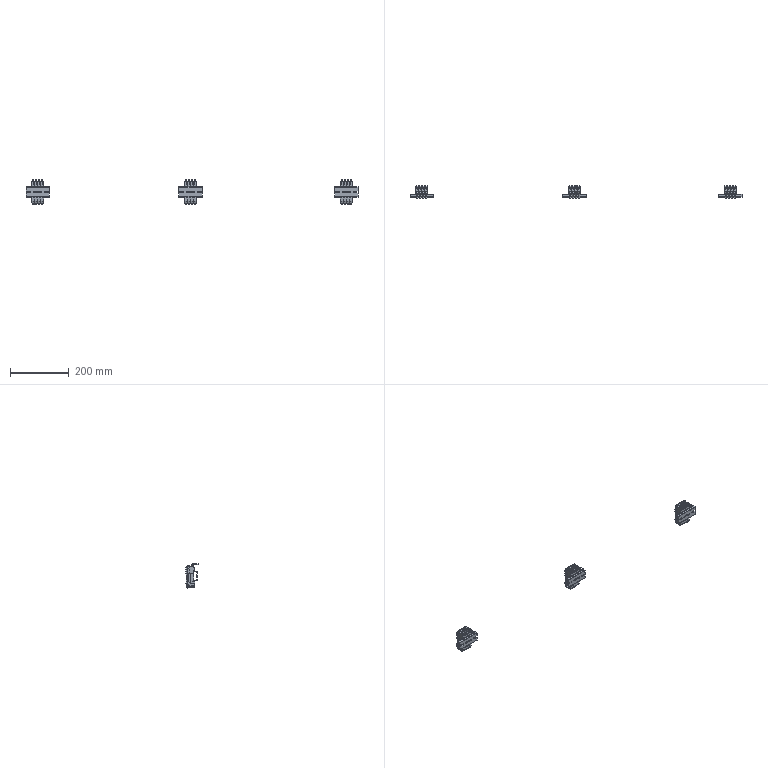Part | NX | 15 solids | 3882 faces | volume 246692 mm3 | plane 2778 | cylinder 864 | cone 108 | spline 96 | torus 36 | commonest cylinder face diameters 2 x108 1.66 x72 0.6 x48 3.628 x48 3.9 x48 1.601 x24